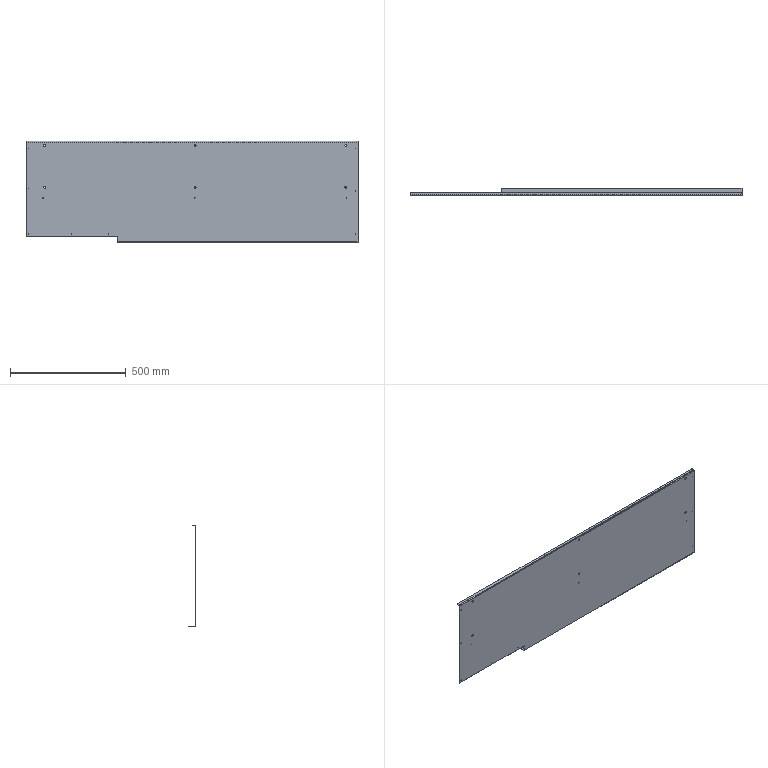Part | NX | features solid 2 | 1 solid | 52 faces | box 1433 x 33 x 437 mm | volume 1325782 mm3 | cylinder 40 | plane 12 | commonest cylinder face diameters 2 x22 8 x14 4 x2 10 x2